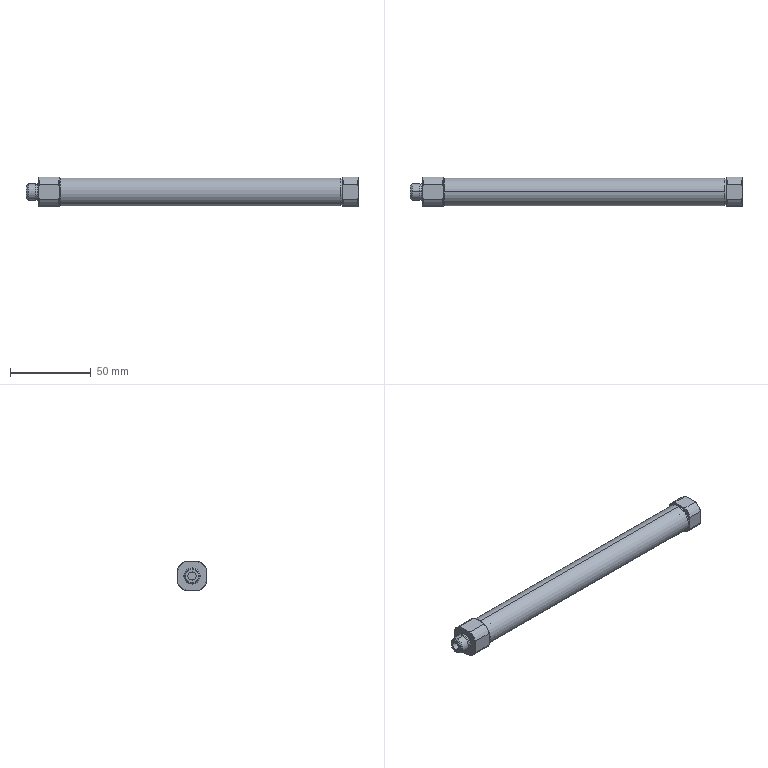Part | STEP file | QA-HI_SBA16x150-SB2-LB_B | 1 solid | 76 faces | box 205 x 18 x 18 mm | volume 13813 mm3 | cylinder 28 | spline 18 | plane 18 | cone 12 | commonest cylinder face diameters 20 x8 4.134 x4 10 x4 16.45 x4 5 x2 8.5 x2